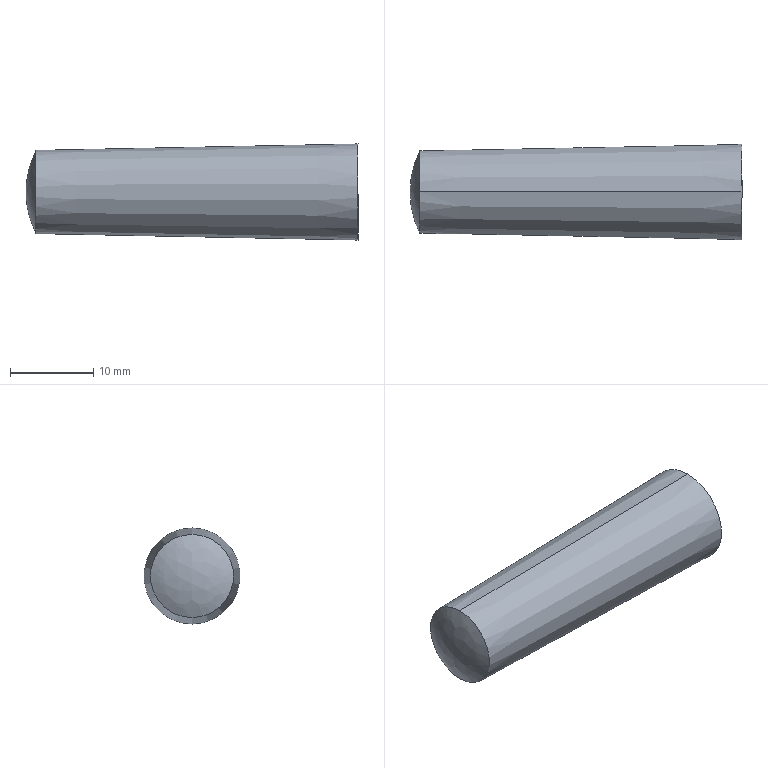Part | SolidWorks | features BaseBody 1, Cut 1 | 1 solid | 4 faces | box 39.9 x 11.548 x 11.548 mm | volume 3582 mm3 | cone 2 | spline 1 | plane 1
STEP:
#1=CARTESIAN_POINT('',(1.2,0.,-5.));
#2=VERTEX_POINT('',#1);
#3=CARTESIAN_POINT('',(1.2,0.,5.));
#4=VERTEX_POINT('',#3);
#5=CARTESIAN_POINT('',(1.2,0.,0.));
#6=DIRECTION('',(1.,0.,0.));
#7=DIRECTION('',(0.,0.,-1.));
#8=AXIS2_PLACEMENT_3D('',#5,#6,#7);
#9=CIRCLE('',#8,5.);
#10=EDGE_CURVE('',#2,#4,#9,.T.);
#11=ORIENTED_EDGE('',*,*,#10,.T.);
#12=CARTESIAN_POINT('',(39.9,0.,5.774));
#13=VERTEX_POINT('',#12);
#14=CARTESIAN_POINT('',(88.8,0.,6.752));
#15=DIRECTION('',(0.9998,0.,0.02));
#16=VECTOR('',#15,1000.);
#17=LINE('',#14,#16);
#18=EDGE_CURVE('',#4,#13,#17,.T.);
#19=ORIENTED_EDGE('',*,*,#18,.T.);
#20=CARTESIAN_POINT('',(39.9,0.,-5.774));
#21=VERTEX_POINT('',#20);
#22=CARTESIAN_POINT('',(39.9,0.,0.));
#23=DIRECTION('',(1.,0.,0.));
#24=DIRECTION('',(0.,0.,1.));
#25=AXIS2_PLACEMENT_3D('',#22,#23,#24);
#26=CIRCLE('',#25,5.774);
#27=EDGE_CURVE('',#21,#13,#26,.T.);
#28=ORIENTED_EDGE('',*,*,#27,.F.);
#29=CARTESIAN_POINT('',(88.8,0.,-6.752));
#30=DIRECTION('',(0.9998,0.,-0.02));
#31=VECTOR('',#30,1000.);
#32=LINE('',#29,#31);
#33=EDGE_CURVE('',#2,#21,#32,.T.);
#34=ORIENTED_EDGE('',*,*,#33,.F.);
#35=EDGE_LOOP('',(#11,#19,#28,#34));
#36=FACE_OUTER_BOUND('',#35,.T.);
#37=CARTESIAN_POINT('',(88.8,0.,0.));
#38=DIRECTION('',(1.,0.,0.));
#39=DIRECTION('',(0.,0.,-1.));
#40=AXIS2_PLACEMENT_3D('',#37,#38,#39);
#41=CONICAL_SURFACE('',#40,6.752,0.02);
#42=ADVANCED_FACE('',(#36),#41,.T.);
#43=ORIENTED_EDGE('',*,*,#18,.F.);
#44=CARTESIAN_POINT('',(1.2,0.,0.));
#45=DIRECTION('',(1.,0.,0.));
#46=DIRECTION('',(0.,0.,-1.));
#47=AXIS2_PLACEMENT_3D('',#44,#45,#46);
#48=CIRCLE('',#47,5.);
#49=EDGE_CURVE('',#4,#2,#48,.T.);
#50=ORIENTED_EDGE('',*,*,#49,.T.);
#51=ORIENTED_EDGE('',*,*,#33,.T.);
#52=CARTESIAN_POINT('',(39.9,0.,0.));
#53=DIRECTION('',(1.,0.,0.));
#54=DIRECTION('',(0.,0.,1.));
#55=AXIS2_PLACEMENT_3D('',#52,#53,#54);
#56=CIRCLE('',#55,5.774);
#57=EDGE_CURVE('',#13,#21,#56,.T.);
#58=ORIENTED_EDGE('',*,*,#57,.F.);
#59=EDGE_LOOP('',(#43,#50,#51,#58));
#60=FACE_OUTER_BOUND('',#59,.T.);
#61=CARTESIAN_POINT('',(88.8,0.,0.));
#62=DIRECTION('',(1.,0.,0.));
#63=DIRECTION('',(0.,0.,-1.));
#64=AXIS2_PLACEMENT_3D('',#61,#62,#63);
#65=CONICAL_SURFACE('',#64,6.752,0.02);
#66=ADVANCED_FACE('',(#60),#65,.T.);
#67=ORIENTED_EDGE('',*,*,#10,.F.);
#68=ORIENTED_EDGE('',*,*,#49,.F.);
#69=EDGE_LOOP('',(#67,#68));
#70=FACE_OUTER_BOUND('',#69,.T.);
#71=CARTESIAN_POINT('',(2.328,5.073,-4.488));
#72=CARTESIAN_POINT('',(0.8407,5.073,-1.608));
#73=CARTESIAN_POINT('',(0.8446,5.073,1.633));
#74=CARTESIAN_POINT('',(2.339,5.073,4.509));
#75=CARTESIAN_POINT('',(0.8286,1.82,-5.262));
#76=CARTESIAN_POINT('',(-0.9153,1.82,-1.886));
#77=CARTESIAN_POINT('',(-0.9107,1.82,1.915));
#78=CARTESIAN_POINT('',(0.8415,1.82,5.287));
#79=CARTESIAN_POINT('',(0.8322,-1.845,-5.26));
#80=CARTESIAN_POINT('',(-0.9111,-1.845,-1.885));
#81=CARTESIAN_POINT('',(-0.9065,-1.845,1.914));
#82=CARTESIAN_POINT('',(0.8451,-1.845,5.285));
#83=CARTESIAN_POINT('',(2.338,-5.094,-4.483));
#84=CARTESIAN_POINT('',(0.8523,-5.094,-1.606));
#85=CARTESIAN_POINT('',(0.8562,-5.094,1.631));
#86=CARTESIAN_POINT('',(2.349,-5.094,4.504));
#87=(BOUNDED_SURFACE()B_SPLINE_SURFACE(3,3,((#71,#72,#73,#74),(#75,#76,#77,#78),(#79,#80,#81,#82),(#83,#84,#85,#86)),.UNSPECIFIED.,.F.,.F.,.F.)B_SPLINE_SURFACE_WITH_KNOTS((4,4),(4,4),(0.,1.),(0.,1.),.UNSPECIFIED.)GEOMETRIC_REPRESENTATION_ITEM()RATIONAL_B_SPLINE_SURFACE(((1.,0.9253,0.9253,1.),(0.9248,0.8557,0.8557,0.9248),(0.9248,0.8557,0.8557,0.9248),(1.,0.9253,0.9253,1.)))REPRESENTATION_ITEM('')SURFACE());
#88=ADVANCED_FACE('',(#70),#87,.T.);
#89=ORIENTED_EDGE('',*,*,#27,.T.);
#90=ORIENTED_EDGE('',*,*,#57,.T.);
#91=EDGE_LOOP('',(#89,#90));
#92=FACE_OUTER_BOUND('',#91,.T.);
#93=CARTESIAN_POINT('',(39.9,-15.929,-0.5818));
#94=DIRECTION('',(-1.,0.,0.));
#95=DIRECTION('',(0.,0.,1.));
#96=AXIS2_PLACEMENT_3D('',#93,#94,#95);
#97=PLANE('',#96);
#98=ADVANCED_FACE('',(#92),#97,.F.);
#99=CLOSED_SHELL('',(#42,#66,#88,#98));
#100=MANIFOLD_SOLID_BREP('',#99);
#101=CARTESIAN_POINT('',(0.,0.,0.));
#102=DIRECTION('',(0.,0.,1.));
#103=DIRECTION('',(1.,0.,0.));
#104=AXIS2_PLACEMENT_3D('',#101,#102,#103);
#105=(LENGTH_UNIT()NAMED_UNIT(*)SI_UNIT(.MILLI.,.METRE.));
#106=UNCERTAINTY_MEASURE_WITH_UNIT(LENGTH_MEASURE(0.00001),#105,'','');
#107=(NAMED_UNIT(*)PLANE_ANGLE_UNIT()SI_UNIT($,.RADIAN.));
#108=(NAMED_UNIT(*)SI_UNIT($,.STERADIAN.)SOLID_ANGLE_UNIT());
#109=(GEOMETRIC_REPRESENTATION_CONTEXT(3)GLOBAL_UNCERTAINTY_ASSIGNED_CONTEXT((#106))GLOBAL_UNIT_ASSIGNED_CONTEXT((#105,#107,#108))REPRESENTATION_CONTEXT('',''));
#110=ADVANCED_BREP_SHAPE_REPRESENTATION('',(#100,#104),#109);